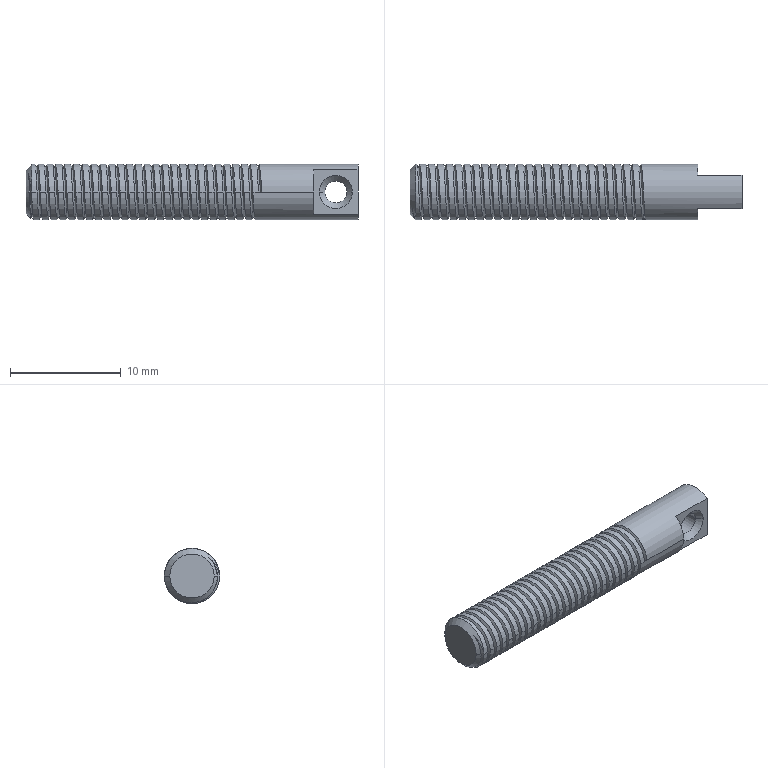Part | NX | 1 solid | 83 faces | box 30 x 5 x 5 mm | volume 537.964 mm3 | cylinder 56 | spline 14 | plane 7 | cone 6 | commonest cylinder face diameters 5 x54 2 x2